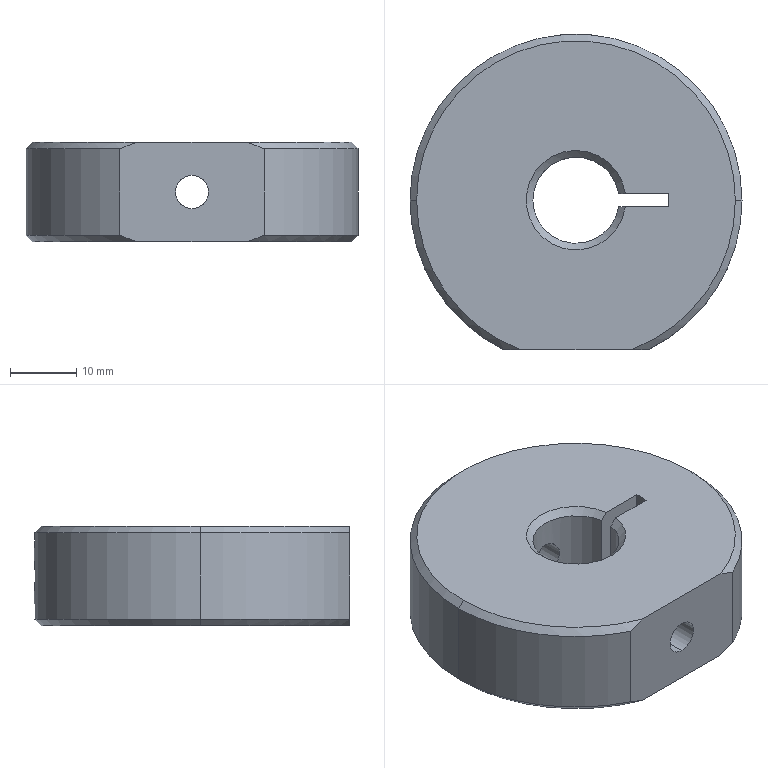Part | STEP file | 11-FG-B01511 | 1 solid | 24 faces | box 50 x 47.5 x 15 mm | volume 25829 mm3 | cylinder 10 | cone 9 | plane 5 | commonest cylinder face diameters 5 x4 50 x3 13 x2 28 x1
STEP:
#1=CARTESIAN_POINT('',(0.,25.,10.));
#2=VERTEX_POINT('',#1);
#3=CARTESIAN_POINT('',(0.,25.,5.));
#4=VERTEX_POINT('',#3);
#5=CARTESIAN_POINT('',(0.,25.,10.));
#6=CARTESIAN_POINT('',(-0.1632,25.,10.));
#7=CARTESIAN_POINT('',(-0.3254,24.998,9.984));
#8=CARTESIAN_POINT('',(-0.648,24.992,9.92));
#9=CARTESIAN_POINT('',(-0.8058,24.987,9.872));
#10=CARTESIAN_POINT('',(-1.107,24.976,9.748));
#11=CARTESIAN_POINT('',(-1.252,24.969,9.67));
#12=CARTESIAN_POINT('',(-1.525,24.954,9.487));
#13=CARTESIAN_POINT('',(-1.651,24.946,9.384));
#14=CARTESIAN_POINT('',(-1.882,24.929,9.154));
#15=CARTESIAN_POINT('',(-1.987,24.921,9.025));
#16=CARTESIAN_POINT('',(-2.169,24.906,8.754));
#17=CARTESIAN_POINT('',(-2.246,24.899,8.61));
#18=CARTESIAN_POINT('',(-2.372,24.887,8.308));
#19=CARTESIAN_POINT('',(-2.42,24.883,8.149));
#20=CARTESIAN_POINT('',(-2.484,24.876,7.829));
#21=CARTESIAN_POINT('',(-2.5,24.875,7.667));
#22=CARTESIAN_POINT('',(-2.5,24.875,7.337));
#23=CARTESIAN_POINT('',(-2.484,24.876,7.174));
#24=CARTESIAN_POINT('',(-2.421,24.883,6.854));
#25=CARTESIAN_POINT('',(-2.373,24.887,6.696));
#26=CARTESIAN_POINT('',(-2.247,24.899,6.393));
#27=CARTESIAN_POINT('',(-2.171,24.906,6.249));
#28=CARTESIAN_POINT('',(-1.99,24.921,5.977));
#29=CARTESIAN_POINT('',(-1.884,24.929,5.849));
#30=CARTESIAN_POINT('',(-1.654,24.946,5.618));
#31=CARTESIAN_POINT('',(-1.528,24.954,5.515));
#32=CARTESIAN_POINT('',(-1.255,24.969,5.332));
#33=CARTESIAN_POINT('',(-1.11,24.976,5.254));
#34=CARTESIAN_POINT('',(-0.6589,24.993,5.067));
#35=CARTESIAN_POINT('',(-0.3305,25.,5.));
#36=CARTESIAN_POINT('',(0.,25.,5.));
#37=B_SPLINE_CURVE_WITH_KNOTS('',3,(#5,#6,#7,#8,#9,#10,#11,#12,#13,#14,#15,#16,#17,#18,#19,#20,#21,#22,#23,#24,#25,#26,#27,#28,#29,#30,#31,#32,#33,#34,#35,#36),.UNSPECIFIED.,.F.,.F.,(4,2,2,2,2,2,2,2,2,2,2,2,2,2,2,4),(0.007821,0.00831,0.008798,0.009287,0.009776,0.01026,0.01075,0.01124,0.01173,0.01222,0.01271,0.0132,0.01369,0.01417,0.01466,0.01564),.UNSPECIFIED.);
#38=EDGE_CURVE('',#2,#4,#37,.T.);
#39=ORIENTED_EDGE('',*,*,#38,.F.);
#40=CARTESIAN_POINT('',(0.,6.5,10.));
#41=VERTEX_POINT('',#40);
#42=CARTESIAN_POINT('',(0.,-22.5,10.));
#43=DIRECTION('',(0.,-1.,0.));
#44=VECTOR('',#43,1000.);
#45=LINE('',#42,#44);
#46=EDGE_CURVE('',#2,#41,#45,.T.);
#47=ORIENTED_EDGE('',*,*,#46,.T.);
#48=CARTESIAN_POINT('',(0.,6.5,5.));
#49=VERTEX_POINT('',#48);
#50=CARTESIAN_POINT('',(0.,6.5,10.));
#51=CARTESIAN_POINT('',(-0.1644,6.5,10.));
#52=CARTESIAN_POINT('',(-0.3308,6.494,9.984));
#53=CARTESIAN_POINT('',(-0.6549,6.469,9.918));
#54=CARTESIAN_POINT('',(-0.8114,6.451,9.87));
#55=CARTESIAN_POINT('',(-1.114,6.406,9.744));
#56=CARTESIAN_POINT('',(-1.259,6.378,9.666));
#57=CARTESIAN_POINT('',(-1.529,6.319,9.485));
#58=CARTESIAN_POINT('',(-1.654,6.287,9.382));
#59=CARTESIAN_POINT('',(-1.885,6.222,9.151));
#60=CARTESIAN_POINT('',(-1.987,6.189,9.025));
#61=CARTESIAN_POINT('',(-2.167,6.129,8.757));
#62=CARTESIAN_POINT('',(-2.245,6.1,8.611));
#63=CARTESIAN_POINT('',(-2.371,6.052,8.309));
#64=CARTESIAN_POINT('',(-2.419,6.033,8.153));
#65=CARTESIAN_POINT('',(-2.483,6.007,7.831));
#66=CARTESIAN_POINT('',(-2.5,6.,7.663));
#67=CARTESIAN_POINT('',(-2.5,6.,7.334));
#68=CARTESIAN_POINT('',(-2.484,6.007,7.17));
#69=CARTESIAN_POINT('',(-2.418,6.033,6.845));
#70=CARTESIAN_POINT('',(-2.37,6.053,6.687));
#71=CARTESIAN_POINT('',(-2.244,6.101,6.386));
#72=CARTESIAN_POINT('',(-2.166,6.129,6.241));
#73=CARTESIAN_POINT('',(-1.984,6.19,5.971));
#74=CARTESIAN_POINT('',(-1.882,6.223,5.846));
#75=CARTESIAN_POINT('',(-1.652,6.288,5.617));
#76=CARTESIAN_POINT('',(-1.525,6.32,5.512));
#77=CARTESIAN_POINT('',(-1.256,6.379,5.332));
#78=CARTESIAN_POINT('',(-1.113,6.406,5.255));
#79=CARTESIAN_POINT('',(-0.8088,6.451,5.129));
#80=CARTESIAN_POINT('',(-0.6508,6.469,5.081));
#81=CARTESIAN_POINT('',(-0.3305,6.494,5.017));
#82=CARTESIAN_POINT('',(-0.1669,6.5,5.));
#83=CARTESIAN_POINT('',(0.,6.5,5.));
#84=B_SPLINE_CURVE_WITH_KNOTS('',3,(#50,#51,#52,#53,#54,#55,#56,#57,#58,#59,#60,#61,#62,#63,#64,#65,#66,#67,#68,#69,#70,#71,#72,#73,#74,#75,#76,#77,#78,#79,#80,#81,#82,#83),.UNSPECIFIED.,.F.,.F.,(4,2,2,2,2,2,2,2,2,2,2,2,2,2,2,2,4),(0.007893,0.008386,0.008879,0.009373,0.009866,0.01036,0.01085,0.01135,0.01184,0.01233,0.01283,0.01332,0.01381,0.0143,0.0148,0.01529,0.01578),.UNSPECIFIED.);
#85=EDGE_CURVE('',#41,#49,#84,.T.);
#86=ORIENTED_EDGE('',*,*,#85,.T.);
#87=CARTESIAN_POINT('',(0.,-22.5,5.));
#88=DIRECTION('',(0.,-1.,0.));
#89=VECTOR('',#88,1000.);
#90=LINE('',#87,#89);
#91=EDGE_CURVE('',#4,#49,#90,.T.);
#92=ORIENTED_EDGE('',*,*,#91,.F.);
#93=EDGE_LOOP('',(#39,#47,#86,#92));
#94=FACE_OUTER_BOUND('',#93,.T.);
#95=CARTESIAN_POINT('',(0.,-22.5,7.5));
#96=DIRECTION('',(0.,-1.,0.));
#97=DIRECTION('',(0.,0.,-1.));
#98=AXIS2_PLACEMENT_3D('',#95,#96,#97);
#99=CYLINDRICAL_SURFACE('',#98,2.5);
#100=ADVANCED_FACE('',(#94),#99,.F.);
#101=CARTESIAN_POINT('',(0.,-6.5,5.));
#102=VERTEX_POINT('',#101);
#103=CARTESIAN_POINT('',(0.,-6.5,10.));
#104=VERTEX_POINT('',#103);
#105=CARTESIAN_POINT('',(0.,-6.5,5.));
#106=CARTESIAN_POINT('',(-0.1669,-6.5,5.));
#107=CARTESIAN_POINT('',(-0.3307,-6.494,5.017));
#108=CARTESIAN_POINT('',(-0.6525,-6.469,5.081));
#109=CARTESIAN_POINT('',(-0.8122,-6.451,5.13));
#110=CARTESIAN_POINT('',(-1.114,-6.406,5.256));
#111=CARTESIAN_POINT('',(-1.257,-6.379,5.333));
#112=CARTESIAN_POINT('',(-1.528,-6.319,5.515));
#113=CARTESIAN_POINT('',(-1.655,-6.287,5.619));
#114=CARTESIAN_POINT('',(-1.997,-6.19,5.962));
#115=CARTESIAN_POINT('',(-2.182,-6.124,6.238));
#116=CARTESIAN_POINT('',(-2.37,-6.053,6.688));
#117=CARTESIAN_POINT('',(-2.419,-6.033,6.847));
#118=CARTESIAN_POINT('',(-2.484,-6.007,7.17));
#119=CARTESIAN_POINT('',(-2.5,-6.,7.334));
#120=CARTESIAN_POINT('',(-2.5,-6.,7.663));
#121=CARTESIAN_POINT('',(-2.483,-6.007,7.831));
#122=CARTESIAN_POINT('',(-2.419,-6.033,8.153));
#123=CARTESIAN_POINT('',(-2.371,-6.053,8.31));
#124=CARTESIAN_POINT('',(-2.244,-6.101,8.614));
#125=CARTESIAN_POINT('',(-2.167,-6.129,8.758));
#126=CARTESIAN_POINT('',(-1.986,-6.19,9.027));
#127=CARTESIAN_POINT('',(-1.882,-6.223,9.154));
#128=CARTESIAN_POINT('',(-1.652,-6.288,9.383));
#129=CARTESIAN_POINT('',(-1.528,-6.319,9.485));
#130=CARTESIAN_POINT('',(-1.258,-6.379,9.667));
#131=CARTESIAN_POINT('',(-1.112,-6.406,9.745));
#132=CARTESIAN_POINT('',(-0.8111,-6.451,9.87));
#133=CARTESIAN_POINT('',(-0.6549,-6.469,9.918));
#134=CARTESIAN_POINT('',(-0.3297,-6.494,9.984));
#135=CARTESIAN_POINT('',(-0.1644,-6.5,10.));
#136=CARTESIAN_POINT('',(0.,-6.5,10.));
#137=B_SPLINE_CURVE_WITH_KNOTS('',3,(#105,#106,#107,#108,#109,#110,#111,#112,#113,#114,#115,#116,#117,#118,#119,#120,#121,#122,#123,#124,#125,#126,#127,#128,#129,#130,#131,#132,#133,#134,#135,#136),.UNSPECIFIED.,.F.,.F.,(4,2,2,2,2,2,2,2,2,2,2,2,2,2,2,4),(0.,0.0004933,0.0009866,0.00148,0.001973,0.00296,0.003453,0.003946,0.00444,0.004933,0.005426,0.00592,0.006413,0.006906,0.0074,0.007893),.UNSPECIFIED.);
#138=EDGE_CURVE('',#102,#104,#137,.T.);
#139=ORIENTED_EDGE('',*,*,#138,.T.);
#140=CARTESIAN_POINT('',(0.,-22.5,10.));
#141=VERTEX_POINT('',#140);
#142=CARTESIAN_POINT('',(0.,-22.5,10.));
#143=DIRECTION('',(0.,-1.,0.));
#144=VECTOR('',#143,1000.);
#145=LINE('',#142,#144);
#146=EDGE_CURVE('',#104,#141,#145,.T.);
#147=ORIENTED_EDGE('',*,*,#146,.T.);
#148=CARTESIAN_POINT('',(0.,-22.5,5.));
#149=VERTEX_POINT('',#148);
#150=CARTESIAN_POINT('',(0.,-22.5,7.5));
#151=DIRECTION('',(0.,-1.,0.));
#152=DIRECTION('',(0.,0.,-1.));
#153=AXIS2_PLACEMENT_3D('',#150,#151,#152);
#154=CIRCLE('',#153,2.5);
#155=EDGE_CURVE('',#141,#149,#154,.T.);
#156=ORIENTED_EDGE('',*,*,#155,.T.);
#157=CARTESIAN_POINT('',(0.,-22.5,5.));
#158=DIRECTION('',(0.,-1.,0.));
#159=VECTOR('',#158,1000.);
#160=LINE('',#157,#159);
#161=EDGE_CURVE('',#102,#149,#160,.T.);
#162=ORIENTED_EDGE('',*,*,#161,.F.);
#163=EDGE_LOOP('',(#139,#147,#156,#162));
#164=FACE_OUTER_BOUND('',#163,.T.);
#165=CARTESIAN_POINT('',(0.,-22.5,7.5));
#166=DIRECTION('',(0.,-1.,0.));
#167=DIRECTION('',(0.,0.,-1.));
#168=AXIS2_PLACEMENT_3D('',#165,#166,#167);
#169=CYLINDRICAL_SURFACE('',#168,2.5);
#170=ADVANCED_FACE('',(#164),#169,.F.);
#171=CARTESIAN_POINT('',(24.,0.,15.));
#172=VERTEX_POINT('',#171);
#173=CARTESIAN_POINT('',(-24.,0.,15.));
#174=VERTEX_POINT('',#173);
#175=CARTESIAN_POINT('',(0.,0.,15.));
#176=DIRECTION('',(0.,0.,1.));
#177=DIRECTION('',(1.,0.,0.));
#178=AXIS2_PLACEMENT_3D('',#175,#176,#177);
#179=CIRCLE('',#178,24.);
#180=EDGE_CURVE('',#172,#174,#179,.T.);
#181=ORIENTED_EDGE('',*,*,#180,.F.);
#182=CARTESIAN_POINT('',(25.,0.,14.));
#183=VERTEX_POINT('',#182);
#184=CARTESIAN_POINT('',(24.,0.,15.));
#185=DIRECTION('',(0.7071,0.,-0.7071));
#186=VECTOR('',#185,1000.);
#187=LINE('',#184,#186);
#188=EDGE_CURVE('',#172,#183,#187,.T.);
#189=ORIENTED_EDGE('',*,*,#188,.T.);
#190=CARTESIAN_POINT('',(-25.,0.,14.));
#191=VERTEX_POINT('',#190);
#192=CARTESIAN_POINT('',(0.,0.,14.));
#193=DIRECTION('',(0.,0.,-1.));
#194=DIRECTION('',(1.,0.,0.));
#195=AXIS2_PLACEMENT_3D('',#192,#193,#194);
#196=CIRCLE('',#195,25.);
#197=EDGE_CURVE('',#191,#183,#196,.T.);
#198=ORIENTED_EDGE('',*,*,#197,.F.);
#199=CARTESIAN_POINT('',(-24.,0.,15.));
#200=DIRECTION('',(-0.7071,0.,-0.7071));
#201=VECTOR('',#200,1000.);
#202=LINE('',#199,#201);
#203=EDGE_CURVE('',#174,#191,#202,.T.);
#204=ORIENTED_EDGE('',*,*,#203,.F.);
#205=EDGE_LOOP('',(#181,#189,#198,#204));
#206=FACE_OUTER_BOUND('',#205,.T.);
#207=CARTESIAN_POINT('',(0.,0.,15.));
#208=DIRECTION('',(0.,0.,-1.));
#209=DIRECTION('',(-1.,0.,0.));
#210=AXIS2_PLACEMENT_3D('',#207,#208,#209);
#211=CONICAL_SURFACE('',#210,24.,0.7854);
#212=ADVANCED_FACE('',(#206),#211,.T.);
#213=CARTESIAN_POINT('',(-8.352,-22.5,15.));
#214=VERTEX_POINT('',#213);
#215=CARTESIAN_POINT('',(0.,0.,15.));
#216=DIRECTION('',(0.,0.,1.));
#217=DIRECTION('',(1.,0.,0.));
#218=AXIS2_PLACEMENT_3D('',#215,#216,#217);
#219=CIRCLE('',#218,24.);
#220=EDGE_CURVE('',#174,#214,#219,.T.);
#221=ORIENTED_EDGE('',*,*,#220,.F.);
#222=ORIENTED_EDGE('',*,*,#203,.T.);
#223=CARTESIAN_POINT('',(-10.897,-22.5,14.));
#224=VERTEX_POINT('',#223);
#225=CARTESIAN_POINT('',(0.,0.,14.));
#226=DIRECTION('',(0.,0.,-1.));
#227=DIRECTION('',(1.,0.,0.));
#228=AXIS2_PLACEMENT_3D('',#225,#226,#227);
#229=CIRCLE('',#228,25.);
#230=EDGE_CURVE('',#224,#191,#229,.T.);
#231=ORIENTED_EDGE('',*,*,#230,.F.);
#232=CARTESIAN_POINT('',(-8.352,-22.5,15.));
#233=CARTESIAN_POINT('',(-9.21,-22.5,14.701));
#234=CARTESIAN_POINT('',(-10.062,-22.5,14.364));
#235=CARTESIAN_POINT('',(-10.897,-22.5,14.));
#236=B_SPLINE_CURVE_WITH_KNOTS('',3,(#232,#233,#234,#235),.UNSPECIFIED.,.F.,.F.,(4,4),(0.06645,0.06918),.UNSPECIFIED.);
#237=EDGE_CURVE('',#214,#224,#236,.T.);
#238=ORIENTED_EDGE('',*,*,#237,.F.);
#239=EDGE_LOOP('',(#221,#222,#231,#238));
#240=FACE_OUTER_BOUND('',#239,.T.);
#241=CARTESIAN_POINT('',(0.,0.,15.));
#242=DIRECTION('',(0.,0.,-1.));
#243=DIRECTION('',(-1.,0.,0.));
#244=AXIS2_PLACEMENT_3D('',#241,#242,#243);
#245=CONICAL_SURFACE('',#244,24.,0.7854);
#246=ADVANCED_FACE('',(#240),#245,.T.);
#247=CARTESIAN_POINT('',(-24.,0.,0.));
#248=VERTEX_POINT('',#247);
#249=CARTESIAN_POINT('',(24.,0.,0.));
#250=VERTEX_POINT('',#249);
#251=CARTESIAN_POINT('',(0.,0.,0.));
#252=DIRECTION('',(0.,0.,-1.));
#253=DIRECTION('',(1.,0.,0.));
#254=AXIS2_PLACEMENT_3D('',#251,#252,#253);
#255=CIRCLE('',#254,24.);
#256=EDGE_CURVE('',#248,#250,#255,.T.);
#257=ORIENTED_EDGE('',*,*,#256,.F.);
#258=CARTESIAN_POINT('',(-25.,0.,1.));
#259=VERTEX_POINT('',#258);
#260=CARTESIAN_POINT('',(-25.,0.,1.));
#261=DIRECTION('',(-0.7071,0.,0.7071));
#262=VECTOR('',#261,1000.);
#263=LINE('',#260,#262);
#264=EDGE_CURVE('',#248,#259,#263,.T.);
#265=ORIENTED_EDGE('',*,*,#264,.T.);
#266=CARTESIAN_POINT('',(25.,0.,1.));
#267=VERTEX_POINT('',#266);
#268=CARTESIAN_POINT('',(0.,0.,1.));
#269=DIRECTION('',(0.,0.,1.));
#270=DIRECTION('',(1.,0.,0.));
#271=AXIS2_PLACEMENT_3D('',#268,#269,#270);
#272=CIRCLE('',#271,25.);
#273=EDGE_CURVE('',#267,#259,#272,.T.);
#274=ORIENTED_EDGE('',*,*,#273,.F.);
#275=CARTESIAN_POINT('',(25.,0.,1.));
#276=DIRECTION('',(0.7071,0.,0.7071));
#277=VECTOR('',#276,1000.);
#278=LINE('',#275,#277);
#279=EDGE_CURVE('',#250,#267,#278,.T.);
#280=ORIENTED_EDGE('',*,*,#279,.F.);
#281=EDGE_LOOP('',(#257,#265,#274,#280));
#282=FACE_OUTER_BOUND('',#281,.T.);
#283=CARTESIAN_POINT('',(0.,0.,1.));
#284=DIRECTION('',(0.,0.,1.));
#285=DIRECTION('',(1.,0.,0.));
#286=AXIS2_PLACEMENT_3D('',#283,#284,#285);
#287=CONICAL_SURFACE('',#286,25.,0.7854);
#288=ADVANCED_FACE('',(#282),#287,.T.);
#289=CARTESIAN_POINT('',(8.352,-22.5,0.));
#290=VERTEX_POINT('',#289);
#291=CARTESIAN_POINT('',(0.,0.,0.));
#292=DIRECTION('',(0.,0.,-1.));
#293=DIRECTION('',(1.,0.,0.));
#294=AXIS2_PLACEMENT_3D('',#291,#292,#293);
#295=CIRCLE('',#294,24.);
#296=EDGE_CURVE('',#250,#290,#295,.T.);
#297=ORIENTED_EDGE('',*,*,#296,.F.);
#298=ORIENTED_EDGE('',*,*,#279,.T.);
#299=CARTESIAN_POINT('',(10.897,-22.5,1.));
#300=VERTEX_POINT('',#299);
#301=CARTESIAN_POINT('',(0.,0.,1.));
#302=DIRECTION('',(0.,0.,1.));
#303=DIRECTION('',(1.,0.,0.));
#304=AXIS2_PLACEMENT_3D('',#301,#302,#303);
#305=CIRCLE('',#304,25.);
#306=EDGE_CURVE('',#300,#267,#305,.T.);
#307=ORIENTED_EDGE('',*,*,#306,.F.);
#308=CARTESIAN_POINT('',(8.352,-22.5,0.));
#309=CARTESIAN_POINT('',(9.21,-22.5,0.2988));
#310=CARTESIAN_POINT('',(10.062,-22.5,0.6359));
#311=CARTESIAN_POINT('',(10.897,-22.5,1.));
#312=B_SPLINE_CURVE_WITH_KNOTS('',3,(#308,#309,#310,#311),.UNSPECIFIED.,.F.,.F.,(4,4),(0.06645,0.06918),.UNSPECIFIED.);
#313=EDGE_CURVE('',#290,#300,#312,.T.);
#314=ORIENTED_EDGE('',*,*,#313,.F.);
#315=EDGE_LOOP('',(#297,#298,#307,#314));
#316=FACE_OUTER_BOUND('',#315,.T.);
#317=CARTESIAN_POINT('',(0.,0.,1.));
#318=DIRECTION('',(0.,0.,1.));
#319=DIRECTION('',(1.,0.,0.));
#320=AXIS2_PLACEMENT_3D('',#317,#318,#319);
#321=CONICAL_SURFACE('',#320,25.,0.7854);
#322=ADVANCED_FACE('',(#316),#321,.T.);
#323=CARTESIAN_POINT('',(-6.5,0.,1.));
#324=VERTEX_POINT('',#323);
#325=CARTESIAN_POINT('',(6.423,1.,1.));
#326=VERTEX_POINT('',#325);
#327=CARTESIAN_POINT('',(0.,0.,1.));
#328=DIRECTION('',(0.,0.,-1.));
#329=DIRECTION('',(1.,0.,0.));
#330=AXIS2_PLACEMENT_3D('',#327,#328,#329);
#331=CIRCLE('',#330,6.5);
#332=EDGE_CURVE('',#324,#326,#331,.T.);
#333=ORIENTED_EDGE('',*,*,#332,.F.);
#334=CARTESIAN_POINT('',(-7.5,0.,0.));
#335=VERTEX_POINT('',#334);
#336=CARTESIAN_POINT('',(-7.5,0.,0.));
#337=DIRECTION('',(-0.7071,0.,-0.7071));
#338=VECTOR('',#337,1000.);
#339=LINE('',#336,#338);
#340=EDGE_CURVE('',#324,#335,#339,.T.);
#341=ORIENTED_EDGE('',*,*,#340,.T.);
#342=CARTESIAN_POINT('',(7.433,1.,0.));
#343=VERTEX_POINT('',#342);
#344=CARTESIAN_POINT('',(0.,0.,0.));
#345=DIRECTION('',(0.,0.,1.));
#346=DIRECTION('',(1.,0.,0.));
#347=AXIS2_PLACEMENT_3D('',#344,#345,#346);
#348=CIRCLE('',#347,7.5);
#349=EDGE_CURVE('',#343,#335,#348,.T.);
#350=ORIENTED_EDGE('',*,*,#349,.F.);
#351=CARTESIAN_POINT('',(6.423,1.,1.));
#352=CARTESIAN_POINT('',(6.595,1.,0.8297));
#353=CARTESIAN_POINT('',(6.767,1.,0.6594));
#354=CARTESIAN_POINT('',(6.939,1.,0.4889));
#355=CARTESIAN_POINT('',(7.104,1.,0.326));
#356=CARTESIAN_POINT('',(7.269,1.,0.163));
#357=CARTESIAN_POINT('',(7.433,1.,0.));
#358=B_SPLINE_CURVE_WITH_KNOTS('',3,(#351,#352,#353,#354,#355,#356,#357),.UNSPECIFIED.,.F.,.F.,(4,3,4),(0.001962,0.002688,0.003383),.UNSPECIFIED.);
#359=EDGE_CURVE('',#326,#343,#358,.T.);
#360=ORIENTED_EDGE('',*,*,#359,.F.);
#361=EDGE_LOOP('',(#333,#341,#350,#360));
#362=FACE_OUTER_BOUND('',#361,.T.);
#363=CARTESIAN_POINT('',(0.,0.,0.));
#364=DIRECTION('',(0.,0.,-1.));
#365=DIRECTION('',(-1.,0.,0.));
#366=AXIS2_PLACEMENT_3D('',#363,#364,#365);
#367=CONICAL_SURFACE('',#366,7.5,0.7854);
#368=ADVANCED_FACE('',(#362),#367,.F.);
#369=CARTESIAN_POINT('',(0.,6.5,5.));
#370=CARTESIAN_POINT('',(0.1669,6.5,5.));
#371=CARTESIAN_POINT('',(0.3307,6.494,5.017));
#372=CARTESIAN_POINT('',(0.6525,6.469,5.081));
#373=CARTESIAN_POINT('',(0.8122,6.451,5.13));
#374=CARTESIAN_POINT('',(1.114,6.406,5.256));
#375=CARTESIAN_POINT('',(1.257,6.379,5.333));
#376=CARTESIAN_POINT('',(1.528,6.319,5.515));
#377=CARTESIAN_POINT('',(1.655,6.287,5.619));
#378=CARTESIAN_POINT('',(1.997,6.19,5.962));
#379=CARTESIAN_POINT('',(2.182,6.124,6.238));
#380=CARTESIAN_POINT('',(2.37,6.053,6.688));
#381=CARTESIAN_POINT('',(2.419,6.033,6.847));
#382=CARTESIAN_POINT('',(2.484,6.007,7.17));
#383=CARTESIAN_POINT('',(2.5,6.,7.334));
#384=CARTESIAN_POINT('',(2.5,6.,7.663));
#385=CARTESIAN_POINT('',(2.483,6.007,7.831));
#386=CARTESIAN_POINT('',(2.419,6.033,8.153));
#387=CARTESIAN_POINT('',(2.371,6.053,8.31));
#388=CARTESIAN_POINT('',(2.244,6.101,8.614));
#389=CARTESIAN_POINT('',(2.167,6.129,8.758));
#390=CARTESIAN_POINT('',(1.986,6.19,9.027));
#391=CARTESIAN_POINT('',(1.882,6.223,9.154));
#392=CARTESIAN_POINT('',(1.652,6.288,9.383));
#393=CARTESIAN_POINT('',(1.528,6.319,9.485));
#394=CARTESIAN_POINT('',(1.258,6.379,9.667));
#395=CARTESIAN_POINT('',(1.112,6.406,9.745));
#396=CARTESIAN_POINT('',(0.8111,6.451,9.87));
#397=CARTESIAN_POINT('',(0.6549,6.469,9.918));
#398=CARTESIAN_POINT('',(0.3297,6.494,9.984));
#399=CARTESIAN_POINT('',(0.1644,6.5,10.));
#400=CARTESIAN_POINT('',(0.,6.5,10.));
#401=B_SPLINE_CURVE_WITH_KNOTS('',3,(#369,#370,#371,#372,#373,#374,#375,#376,#377,#378,#379,#380,#381,#382,#383,#384,#385,#386,#387,#388,#389,#390,#391,#392,#393,#394,#395,#396,#397,#398,#399,#400),.UNSPECIFIED.,.F.,.F.,(4,2,2,2,2,2,2,2,2,2,2,2,2,2,2,4),(0.,0.0004933,0.0009866,0.00148,0.001973,0.00296,0.003453,0.003946,0.00444,0.004933,0.005426,0.00592,0.006413,0.006906,0.0074,0.007893),.UNSPECIFIED.);
#402=EDGE_CURVE('',#49,#41,#401,.T.);
#403=ORIENTED_EDGE('',*,*,#402,.F.);
#404=ORIENTED_EDGE('',*,*,#85,.F.);
#405=EDGE_LOOP('',(#403,#404));
#406=FACE_BOUND('',#405,.T.);
#407=CARTESIAN_POINT('',(6.423,1.,14.));
#408=VERTEX_POINT('',#407);
#409=CARTESIAN_POINT('',(-6.5,0.,14.));
#410=VERTEX_POINT('',#409);
#411=CARTESIAN_POINT('',(0.,0.,14.));
#412=DIRECTION('',(0.,0.,1.));
#413=DIRECTION('',(1.,0.,0.));
#414=AXIS2_PLACEMENT_3D('',#411,#412,#413);
#415=CIRCLE('',#414,6.5);
#416=EDGE_CURVE('',#408,#410,#415,.T.);
#417=ORIENTED_EDGE('',*,*,#416,.T.);
#418=CARTESIAN_POINT('',(-6.5,0.,15.));
#419=DIRECTION('',(0.,0.,-1.));
#420=VECTOR('',#419,1000.);
#421=LINE('',#418,#420);
#422=EDGE_CURVE('',#410,#324,#421,.T.);
#423=ORIENTED_EDGE('',*,*,#422,.T.);
#424=ORIENTED_EDGE('',*,*,#332,.T.);
#425=CARTESIAN_POINT('',(6.423,1.,19.));
#426=DIRECTION('',(0.,0.,-1.));
#427=VECTOR('',#426,1000.);
#428=LINE('',#425,#427);
#429=EDGE_CURVE('',#408,#326,#428,.T.);
#430=ORIENTED_EDGE('',*,*,#429,.F.);
#431=EDGE_LOOP('',(#417,#423,#424,#430));
#432=FACE_OUTER_BOUND('',#431,.T.);
#433=CARTESIAN_POINT('',(0.,0.,15.));
#434=DIRECTION('',(0.,0.,-1.));
#435=DIRECTION('',(-1.,0.,0.));
#436=AXIS2_PLACEMENT_3D('',#433,#434,#435);
#437=CYLINDRICAL_SURFACE('',#436,6.5);
#438=ADVANCED_FACE('',(#406,#432),#437,.F.);
#439=CARTESIAN_POINT('',(0.,25.,5.));
#440=CARTESIAN_POINT('',(0.1653,25.,5.));
#441=CARTESIAN_POINT('',(0.3278,24.998,5.016));
#442=CARTESIAN_POINT('',(0.6475,24.992,5.08));
#443=CARTESIAN_POINT('',(0.8063,24.987,5.128));
#444=CARTESIAN_POINT('',(1.109,24.976,5.253));
#445=CARTESIAN_POINT('',(1.253,24.969,5.33));
#446=CARTESIAN_POINT('',(1.524,24.954,5.512));
#447=CARTESIAN_POINT('',(1.653,24.946,5.617));
#448=CARTESIAN_POINT('',(1.883,24.929,5.848));
#449=CARTESIAN_POINT('',(1.987,24.921,5.974));
#450=CARTESIAN_POINT('',(2.17,24.906,6.247));
#451=CARTESIAN_POINT('',(2.247,24.899,6.392));
#452=CARTESIAN_POINT('',(2.372,24.887,6.693));
#453=CARTESIAN_POINT('',(2.42,24.883,6.851));
#454=CARTESIAN_POINT('',(2.484,24.876,7.174));
#455=CARTESIAN_POINT('',(2.5,24.875,7.336));
#456=CARTESIAN_POINT('',(2.5,24.875,7.662));
#457=CARTESIAN_POINT('',(2.484,24.876,7.828));
#458=CARTESIAN_POINT('',(2.42,24.883,8.149));
#459=CARTESIAN_POINT('',(2.373,24.887,8.305));
#460=CARTESIAN_POINT('',(2.247,24.899,8.607));
#461=CARTESIAN_POINT('',(2.169,24.906,8.754));
#462=CARTESIAN_POINT('',(1.988,24.921,9.025));
#463=CARTESIAN_POINT('',(1.885,24.929,9.151));
#464=CARTESIAN_POINT('',(1.651,24.946,9.384));
#465=CARTESIAN_POINT('',(1.525,24.954,9.488));
#466=CARTESIAN_POINT('',(1.254,24.969,9.669));
#467=CARTESIAN_POINT('',(1.108,24.976,9.747));
#468=CARTESIAN_POINT('',(0.8054,24.987,9.872));
#469=CARTESIAN_POINT('',(0.6496,24.992,9.92));
#470=CARTESIAN_POINT('',(0.329,24.998,9.984));
#471=CARTESIAN_POINT('',(0.1632,25.,10.));
#472=CARTESIAN_POINT('',(0.,25.,10.));
#473=B_SPLINE_CURVE_WITH_KNOTS('',3,(#439,#440,#441,#442,#443,#444,#445,#446,#447,#448,#449,#450,#451,#452,#453,#454,#455,#456,#457,#458,#459,#460,#461,#462,#463,#464,#465,#466,#467,#468,#469,#470,#471,#472),.UNSPECIFIED.,.F.,.F.,(4,2,2,2,2,2,2,2,2,2,2,2,2,2,2,2,4),(0.,0.0004888,0.0009776,0.001466,0.001955,0.002444,0.002933,0.003422,0.003911,0.004399,0.004888,0.005377,0.005866,0.006355,0.006843,0.007332,0.007821),.UNSPECIFIED.);
#474=EDGE_CURVE('',#4,#2,#473,.T.);
#475=ORIENTED_EDGE('',*,*,#474,.T.);
#476=ORIENTED_EDGE('',*,*,#38,.T.);
#477=EDGE_LOOP('',(#475,#476));
#478=FACE_BOUND('',#477,.T.);
#479=ORIENTED_EDGE('',*,*,#197,.T.);
#480=CARTESIAN_POINT('',(25.,0.,15.));
#481=DIRECTION('',(0.,0.,-1.));
#482=VECTOR('',#481,1000.);
#483=LINE('',#480,#482);
#484=EDGE_CURVE('',#183,#267,#483,.T.);
#485=ORIENTED_EDGE('',*,*,#484,.T.);
#486=ORIENTED_EDGE('',*,*,#273,.T.);
#487=CARTESIAN_POINT('',(-25.,0.,15.));
#488=DIRECTION('',(0.,0.,-1.));
#489=VECTOR('',#488,1000.);
#490=LINE('',#487,#489);
#491=EDGE_CURVE('',#191,#259,#490,.T.);
#492=ORIENTED_EDGE('',*,*,#491,.F.);
#493=EDGE_LOOP('',(#479,#485,#486,#492));
#494=FACE_OUTER_BOUND('',#493,.T.);
#495=CARTESIAN_POINT('',(0.,0.,15.));
#496=DIRECTION('',(0.,0.,-1.));
#497=DIRECTION('',(-1.,0.,0.));
#498=AXIS2_PLACEMENT_3D('',#495,#496,#497);
#499=CYLINDRICAL_SURFACE('',#498,25.);
#500=ADVANCED_FACE('',(#478,#494),#499,.T.);
#501=ORIENTED_EDGE('',*,*,#230,.T.);
#502=ORIENTED_EDGE('',*,*,#491,.T.);
#503=CARTESIAN_POINT('',(-10.897,-22.5,1.));
#504=VERTEX_POINT('',#503);
#505=CARTESIAN_POINT('',(0.,0.,1.));
#506=DIRECTION('',(0.,0.,1.));
#507=DIRECTION('',(1.,0.,0.));
#508=AXIS2_PLACEMENT_3D('',#505,#506,#507);
#509=CIRCLE('',#508,25.);
#510=EDGE_CURVE('',#259,#504,#509,.T.);
#511=ORIENTED_EDGE('',*,*,#510,.T.);
#512=CARTESIAN_POINT('',(-10.897,-22.5,15.));
#513=DIRECTION('',(0.,0.,1.));
#514=VECTOR('',#513,1000.);
#515=LINE('',#512,#514);
#516=EDGE_CURVE('',#504,#224,#515,.T.);
#517=ORIENTED_EDGE('',*,*,#516,.T.);
#518=EDGE_LOOP('',(#501,#502,#511,#517));
#519=FACE_OUTER_BOUND('',#518,.T.);
#520=CARTESIAN_POINT('',(0.,0.,15.));
#521=DIRECTION('',(0.,0.,-1.));
#522=DIRECTION('',(-1.,0.,0.));
#523=AXIS2_PLACEMENT_3D('',#520,#521,#522);
#524=CYLINDRICAL_SURFACE('',#523,25.);
#525=ADVANCED_FACE('',(#519),#524,.T.);
#526=ORIENTED_EDGE('',*,*,#313,.T.);
#527=CARTESIAN_POINT('',(10.897,-22.5,14.));
#528=VERTEX_POINT('',#527);
#529=CARTESIAN_POINT('',(10.897,-22.5,15.));
#530=DIRECTION('',(0.,0.,-1.));
#531=VECTOR('',#530,1000.);
#532=LINE('',#529,#531);
#533=EDGE_CURVE('',#528,#300,#532,.T.);
#534=ORIENTED_EDGE('',*,*,#533,.F.);
#535=CARTESIAN_POINT('',(8.352,-22.5,15.));
#536=VERTEX_POINT('',#535);
#537=CARTESIAN_POINT('',(10.897,-22.5,14.));
#538=CARTESIAN_POINT('',(10.061,-22.5,14.365));
#539=CARTESIAN_POINT('',(9.213,-22.5,14.7));
#540=CARTESIAN_POINT('',(8.352,-22.5,15.));
#541=B_SPLINE_CURVE_WITH_KNOTS('',3,(#537,#538,#539,#540),.UNSPECIFIED.,.F.,.F.,(4,4),(0.04668,0.04942),.UNSPECIFIED.);
#542=EDGE_CURVE('',#528,#536,#541,.T.);
#543=ORIENTED_EDGE('',*,*,#542,.T.);
#544=CARTESIAN_POINT('',(-21.698,-22.5,15.));
#545=DIRECTION('',(-1.,0.,0.));
#546=VECTOR('',#545,1000.);
#547=LINE('',#544,#546);
#548=EDGE_CURVE('',#536,#214,#547,.T.);
#549=ORIENTED_EDGE('',*,*,#548,.T.);
#550=ORIENTED_EDGE('',*,*,#237,.T.);
#551=ORIENTED_EDGE('',*,*,#516,.F.);
#552=CARTESIAN_POINT('',(-8.352,-22.5,0.));
#553=VERTEX_POINT('',#552);
#554=CARTESIAN_POINT('',(-10.897,-22.5,1.));
#555=CARTESIAN_POINT('',(-10.061,-22.5,0.6355));
#556=CARTESIAN_POINT('',(-9.213,-22.5,0.2998));
#557=CARTESIAN_POINT('',(-8.352,-22.5,0.));
#558=B_SPLINE_CURVE_WITH_KNOTS('',3,(#554,#555,#556,#557),.UNSPECIFIED.,.F.,.F.,(4,4),(0.04668,0.04942),.UNSPECIFIED.);
#559=EDGE_CURVE('',#504,#553,#558,.T.);
#560=ORIENTED_EDGE('',*,*,#559,.T.);
#561=CARTESIAN_POINT('',(-21.698,-22.5,0.));
#562=DIRECTION('',(-1.,0.,0.));
#563=VECTOR('',#562,1000.);
#564=LINE('',#561,#563);
#565=EDGE_CURVE('',#290,#553,#564,.T.);
#566=ORIENTED_EDGE('',*,*,#565,.F.);
#567=EDGE_LOOP('',(#526,#534,#543,#549,#550,#551,#560,#566));
#568=FACE_OUTER_BOUND('',#567,.T.);
#569=CARTESIAN_POINT('',(0.,-22.5,7.5));
#570=DIRECTION('',(0.,-1.,0.));
#571=DIRECTION('',(0.,0.,-1.));
#572=AXIS2_PLACEMENT_3D('',#569,#570,#571);
#573=CIRCLE('',#572,2.5);
#574=EDGE_CURVE('',#149,#141,#573,.T.);
#575=ORIENTED_EDGE('',*,*,#574,.F.);
#576=ORIENTED_EDGE('',*,*,#155,.F.);
#577=EDGE_LOOP('',(#575,#576));
#578=FACE_BOUND('',#577,.T.);
#579=CARTESIAN_POINT('',(-21.698,-22.5,0.));
#580=DIRECTION('',(0.,1.,0.));
#581=DIRECTION('',(0.,0.,1.));
#582=AXIS2_PLACEMENT_3D('',#579,#580,#581);
#583=PLANE('',#582);
#584=ADVANCED_FACE('',(#568,#578),#583,.F.);
#585=CARTESIAN_POINT('',(7.433,-1.,15.));
#586=VERTEX_POINT('',#585);
#587=CARTESIAN_POINT('',(13.964,-1.,15.));
#588=VERTEX_POINT('',#587);
#589=CARTESIAN_POINT('',(0.,-1.,15.));
#590=DIRECTION('',(1.,0.,0.));
#591=VECTOR('',#590,1000.);
#592=LINE('',#589,#591);
#593=EDGE_CURVE('',#586,#588,#592,.T.);
#594=ORIENTED_EDGE('',*,*,#593,.F.);
#595=CARTESIAN_POINT('',(7.433,1.,15.));
#596=VERTEX_POINT('',#595);
#597=CARTESIAN_POINT('',(0.,0.,15.));
#598=DIRECTION('',(0.,0.,-1.));
#599=DIRECTION('',(1.,0.,0.));
#600=AXIS2_PLACEMENT_3D('',#597,#598,#599);
#601=CIRCLE('',#600,7.5);
#602=EDGE_CURVE('',#586,#596,#601,.T.);
#603=ORIENTED_EDGE('',*,*,#602,.T.);
#604=CARTESIAN_POINT('',(13.964,1.,15.));
#605=VERTEX_POINT('',#604);
#606=CARTESIAN_POINT('',(0.,1.,15.));
#607=DIRECTION('',(-1.,0.,0.));
#608=VECTOR('',#607,1000.);
#609=LINE('',#606,#608);
#610=EDGE_CURVE('',#605,#596,#609,.T.);
#611=ORIENTED_EDGE('',*,*,#610,.F.);
#612=CARTESIAN_POINT('',(0.,0.,15.));
#613=DIRECTION('',(0.,0.,1.));
#614=DIRECTION('',(1.,0.,0.));
#615=AXIS2_PLACEMENT_3D('',#612,#613,#614);
#616=CIRCLE('',#615,14.);
#617=EDGE_CURVE('',#588,#605,#616,.T.);
#618=ORIENTED_EDGE('',*,*,#617,.F.);
#619=EDGE_LOOP('',(#594,#603,#611,#618));
#620=FACE_BOUND('',#619,.T.);
#621=ORIENTED_EDGE('',*,*,#548,.F.);
#622=CARTESIAN_POINT('',(0.,0.,15.));
#623=DIRECTION('',(0.,0.,1.));
#624=DIRECTION('',(1.,0.,0.));
#625=AXIS2_PLACEMENT_3D('',#622,#623,#624);
#626=CIRCLE('',#625,24.);
#627=EDGE_CURVE('',#536,#172,#626,.T.);
#628=ORIENTED_EDGE('',*,*,#627,.T.);
#629=ORIENTED_EDGE('',*,*,#180,.T.);
#630=ORIENTED_EDGE('',*,*,#220,.T.);
#631=EDGE_LOOP('',(#621,#628,#629,#630));
#632=FACE_OUTER_BOUND('',#631,.T.);
#633=CARTESIAN_POINT('',(0.,0.,15.));
#634=DIRECTION('',(0.,0.,1.));
#635=DIRECTION('',(1.,0.,0.));
#636=AXIS2_PLACEMENT_3D('',#633,#634,#635);
#637=PLANE('',#636);
#638=ADVANCED_FACE('',(#620,#632),#637,.T.);
#639=ORIENTED_EDGE('',*,*,#349,.T.);
#640=CARTESIAN_POINT('',(7.433,-1.,0.));
#641=VERTEX_POINT('',#640);
#642=CARTESIAN_POINT('',(0.,0.,0.));
#643=DIRECTION('',(0.,0.,1.));
#644=DIRECTION('',(1.,0.,0.));
#645=AXIS2_PLACEMENT_3D('',#642,#643,#644);
#646=CIRCLE('',#645,7.5);
#647=EDGE_CURVE('',#335,#641,#646,.T.);
#648=ORIENTED_EDGE('',*,*,#647,.T.);
#649=CARTESIAN_POINT('',(13.964,-1.,0.));
#650=VERTEX_POINT('',#649);
#651=CARTESIAN_POINT('',(6.423,-1.,0.));
#652=DIRECTION('',(-1.,0.,0.));
#653=VECTOR('',#652,1000.);
#654=LINE('',#651,#653);
#655=EDGE_CURVE('',#650,#641,#654,.T.);
#656=ORIENTED_EDGE('',*,*,#655,.F.);
#657=CARTESIAN_POINT('',(13.964,1.,0.));
#658=VERTEX_POINT('',#657);
#659=CARTESIAN_POINT('',(0.,0.,0.));
#660=DIRECTION('',(0.,0.,-1.));
#661=DIRECTION('',(-1.,0.,0.));
#662=AXIS2_PLACEMENT_3D('',#659,#660,#661);
#663=CIRCLE('',#662,14.);
#664=EDGE_CURVE('',#658,#650,#663,.T.);
#665=ORIENTED_EDGE('',*,*,#664,.F.);
#666=CARTESIAN_POINT('',(6.423,1.,0.));
#667=DIRECTION('',(1.,0.,0.));
#668=VECTOR('',#667,1000.);
#669=LINE('',#666,#668);
#670=EDGE_CURVE('',#343,#658,#669,.T.);
#671=ORIENTED_EDGE('',*,*,#670,.F.);
#672=EDGE_LOOP('',(#639,#648,#656,#665,#671));
#673=FACE_BOUND('',#672,.T.);
#674=CARTESIAN_POINT('',(0.,0.,0.));
#675=DIRECTION('',(0.,0.,-1.));
#676=DIRECTION('',(1.,0.,0.));
#677=AXIS2_PLACEMENT_3D('',#674,#675,#676);
#678=CIRCLE('',#677,24.);
#679=EDGE_CURVE('',#553,#248,#678,.T.);
#680=ORIENTED_EDGE('',*,*,#679,.T.);
#681=ORIENTED_EDGE('',*,*,#256,.T.);
#682=ORIENTED_EDGE('',*,*,#296,.T.);
#683=ORIENTED_EDGE('',*,*,#565,.T.);
#684=EDGE_LOOP('',(#680,#681,#682,#683));
#685=FACE_OUTER_BOUND('',#684,.T.);
#686=CARTESIAN_POINT('',(0.,0.,0.));
#687=DIRECTION('',(0.,0.,1.));
#688=DIRECTION('',(1.,0.,0.));
#689=AXIS2_PLACEMENT_3D('',#686,#687,#688);
#690=PLANE('',#689);
#691=ADVANCED_FACE('',(#673,#685),#690,.F.);
#692=ORIENTED_EDGE('',*,*,#484,.F.);
#693=CARTESIAN_POINT('',(0.,0.,14.));
#694=DIRECTION('',(0.,0.,-1.));
#695=DIRECTION('',(1.,0.,0.));
#696=AXIS2_PLACEMENT_3D('',#693,#694,#695);
#697=CIRCLE('',#696,25.);
#698=EDGE_CURVE('',#183,#528,#697,.T.);
#699=ORIENTED_EDGE('',*,*,#698,.T.);
#700=ORIENTED_EDGE('',*,*,#533,.T.);
#701=ORIENTED_EDGE('',*,*,#306,.T.);
#702=EDGE_LOOP('',(#692,#699,#700,#701));
#703=FACE_OUTER_BOUND('',#702,.T.);
#704=CARTESIAN_POINT('',(0.,0.,15.));
#705=DIRECTION('',(0.,0.,-1.));
#706=DIRECTION('',(-1.,0.,0.));
#707=AXIS2_PLACEMENT_3D('',#704,#705,#706);
#708=CYLINDRICAL_SURFACE('',#707,25.);
#709=ADVANCED_FACE('',(#703),#708,.T.);
#710=ORIENTED_EDGE('',*,*,#422,.F.);
#711=CARTESIAN_POINT('',(6.423,-1.,14.));
#712=VERTEX_POINT('',#711);
#713=CARTESIAN_POINT('',(0.,0.,14.));
#714=DIRECTION('',(0.,0.,1.));
#715=DIRECTION('',(1.,0.,0.));
#716=AXIS2_PLACEMENT_3D('',#713,#714,#715);
#717=CIRCLE('',#716,6.5);
#718=EDGE_CURVE('',#410,#712,#717,.T.);
#719=ORIENTED_EDGE('',*,*,#718,.T.);
#720=CARTESIAN_POINT('',(6.423,-1.,1.));
#721=VERTEX_POINT('',#720);
#722=CARTESIAN_POINT('',(6.423,-1.,19.));
#723=DIRECTION('',(0.,0.,-1.));
#724=VECTOR('',#723,1000.);
#725=LINE('',#722,#724);
#726=EDGE_CURVE('',#712,#721,#725,.T.);
#727=ORIENTED_EDGE('',*,*,#726,.T.);
#728=CARTESIAN_POINT('',(0.,0.,1.));
#729=DIRECTION('',(0.,0.,-1.));
#730=DIRECTION('',(1.,0.,0.));
#731=AXIS2_PLACEMENT_3D('',#728,#729,#730);
#732=CIRCLE('',#731,6.5);
#733=EDGE_CURVE('',#721,#324,#732,.T.);
#734=ORIENTED_EDGE('',*,*,#733,.T.);
#735=EDGE_LOOP('',(#710,#719,#727,#734));
#736=FACE_OUTER_BOUND('',#735,.T.);
#737=ORIENTED_EDGE('',*,*,#138,.F.);
#738=CARTESIAN_POINT('',(0.,-6.5,10.));
#739=CARTESIAN_POINT('',(0.1644,-6.5,10.));
#740=CARTESIAN_POINT('',(0.3308,-6.494,9.984));
#741=CARTESIAN_POINT('',(0.6549,-6.469,9.918));
#742=CARTESIAN_POINT('',(0.8114,-6.451,9.87));
#743=CARTESIAN_POINT('',(1.114,-6.406,9.744));
#744=CARTESIAN_POINT('',(1.259,-6.378,9.666));
#745=CARTESIAN_POINT('',(1.529,-6.319,9.485));
#746=CARTESIAN_POINT('',(1.654,-6.287,9.382));
#747=CARTESIAN_POINT('',(1.885,-6.222,9.151));
#748=CARTESIAN_POINT('',(1.987,-6.189,9.025));
#749=CARTESIAN_POINT('',(2.167,-6.129,8.757));
#750=CARTESIAN_POINT('',(2.245,-6.1,8.611));
#751=CARTESIAN_POINT('',(2.371,-6.052,8.309));
#752=CARTESIAN_POINT('',(2.419,-6.033,8.153));
#753=CARTESIAN_POINT('',(2.483,-6.007,7.831));
#754=CARTESIAN_POINT('',(2.5,-6.,7.663));
#755=CARTESIAN_POINT('',(2.5,-6.,7.334));
#756=CARTESIAN_POINT('',(2.484,-6.007,7.17));
#757=CARTESIAN_POINT('',(2.418,-6.033,6.845));
#758=CARTESIAN_POINT('',(2.37,-6.053,6.687));
#759=CARTESIAN_POINT('',(2.244,-6.101,6.386));
#760=CARTESIAN_POINT('',(2.166,-6.129,6.241));
#761=CARTESIAN_POINT('',(1.984,-6.19,5.971));
#762=CARTESIAN_POINT('',(1.882,-6.223,5.846));
#763=CARTESIAN_POINT('',(1.652,-6.288,5.617));
#764=CARTESIAN_POINT('',(1.525,-6.32,5.512));
#765=CARTESIAN_POINT('',(1.256,-6.379,5.332));
#766=CARTESIAN_POINT('',(1.113,-6.406,5.255));
#767=CARTESIAN_POINT('',(0.8088,-6.451,5.129));
#768=CARTESIAN_POINT('',(0.6508,-6.469,5.081));
#769=CARTESIAN_POINT('',(0.3305,-6.494,5.017));
#770=CARTESIAN_POINT('',(0.1669,-6.5,5.));
#771=CARTESIAN_POINT('',(0.,-6.5,5.));
#772=B_SPLINE_CURVE_WITH_KNOTS('',3,(#738,#739,#740,#741,#742,#743,#744,#745,#746,#747,#748,#749,#750,#751,#752,#753,#754,#755,#756,#757,#758,#759,#760,#761,#762,#763,#764,#765,#766,#767,#768,#769,#770,#771),.UNSPECIFIED.,.F.,.F.,(4,2,2,2,2,2,2,2,2,2,2,2,2,2,2,2,4),(0.007893,0.008386,0.008879,0.009373,0.009866,0.01036,0.01085,0.01135,0.01184,0.01233,0.01283,0.01332,0.01381,0.0143,0.0148,0.01529,0.01578),.UNSPECIFIED.);
#773=EDGE_CURVE('',#104,#102,#772,.T.);
#774=ORIENTED_EDGE('',*,*,#773,.F.);
#775=EDGE_LOOP('',(#737,#774));
#776=FACE_BOUND('',#775,.T.);
#777=CARTESIAN_POINT('',(0.,0.,15.));
#778=DIRECTION('',(0.,0.,-1.));
#779=DIRECTION('',(-1.,0.,0.));
#780=AXIS2_PLACEMENT_3D('',#777,#778,#779);
#781=CYLINDRICAL_SURFACE('',#780,6.5);
#782=ADVANCED_FACE('',(#736,#776),#781,.F.);
#783=ORIENTED_EDGE('',*,*,#340,.F.);
#784=ORIENTED_EDGE('',*,*,#733,.F.);
#785=CARTESIAN_POINT('',(7.433,-1.,0.));
#786=CARTESIAN_POINT('',(7.269,-1.,0.163));
#787=CARTESIAN_POINT('',(7.104,-1.,0.326));
#788=CARTESIAN_POINT('',(6.939,-1.,0.4889));
#789=CARTESIAN_POINT('',(6.767,-1.,0.6594));
#790=CARTESIAN_POINT('',(6.595,-1.,0.8297));
#791=CARTESIAN_POINT('',(6.423,-1.,1.));
#792=B_SPLINE_CURVE_WITH_KNOTS('',3,(#785,#786,#787,#788,#789,#790,#791),.UNSPECIFIED.,.F.,.F.,(4,3,4),(0.001994,0.002688,0.003415),.UNSPECIFIED.);
#793=EDGE_CURVE('',#641,#721,#792,.T.);
#794=ORIENTED_EDGE('',*,*,#793,.F.);
#795=ORIENTED_EDGE('',*,*,#647,.F.);
#796=EDGE_LOOP('',(#783,#784,#794,#795));
#797=FACE_OUTER_BOUND('',#796,.T.);
#798=CARTESIAN_POINT('',(0.,0.,0.));
#799=DIRECTION('',(0.,0.,-1.));
#800=DIRECTION('',(-1.,0.,0.));
#801=AXIS2_PLACEMENT_3D('',#798,#799,#800);
#802=CONICAL_SURFACE('',#801,7.5,0.7854);
#803=ADVANCED_FACE('',(#797),#802,.F.);
#804=CARTESIAN_POINT('',(6.423,-1.,14.));
#805=CARTESIAN_POINT('',(6.466,-1.,14.043));
#806=CARTESIAN_POINT('',(6.51,-1.,14.086));
#807=CARTESIAN_POINT('',(6.553,-1.,14.129));
#808=CARTESIAN_POINT('',(6.847,-1.,14.419));
#809=CARTESIAN_POINT('',(7.14,-1.,14.71));
#810=CARTESIAN_POINT('',(7.433,-1.,15.));
#811=B_SPLINE_CURVE_WITH_KNOTS('',3,(#804,#805,#806,#807,#808,#809,#810),.UNSPECIFIED.,.F.,.F.,(4,3,4),(0.002505,0.002688,0.003926),.UNSPECIFIED.);
#812=EDGE_CURVE('',#712,#586,#811,.T.);
#813=ORIENTED_EDGE('',*,*,#812,.F.);
#814=ORIENTED_EDGE('',*,*,#718,.F.);
#815=ORIENTED_EDGE('',*,*,#416,.F.);
#816=CARTESIAN_POINT('',(7.433,1.,15.));
#817=CARTESIAN_POINT('',(7.14,1.,14.71));
#818=CARTESIAN_POINT('',(6.847,1.,14.419));
#819=CARTESIAN_POINT('',(6.553,1.,14.129));
#820=CARTESIAN_POINT('',(6.51,1.,14.086));
#821=CARTESIAN_POINT('',(6.466,1.,14.043));
#822=CARTESIAN_POINT('',(6.423,1.,14.));
#823=B_SPLINE_CURVE_WITH_KNOTS('',3,(#816,#817,#818,#819,#820,#821,#822),.UNSPECIFIED.,.F.,.F.,(4,3,4),(0.00145,0.002688,0.002872),.UNSPECIFIED.);
#824=EDGE_CURVE('',#596,#408,#823,.T.);
#825=ORIENTED_EDGE('',*,*,#824,.F.);
#826=ORIENTED_EDGE('',*,*,#602,.F.);
#827=EDGE_LOOP('',(#813,#814,#815,#825,#826));
#828=FACE_OUTER_BOUND('',#827,.T.);
#829=CARTESIAN_POINT('',(0.,0.,14.));
#830=DIRECTION('',(0.,0.,1.));
#831=DIRECTION('',(1.,0.,0.));
#832=AXIS2_PLACEMENT_3D('',#829,#830,#831);
#833=CONICAL_SURFACE('',#832,6.5,0.7854);
#834=ADVANCED_FACE('',(#828),#833,.F.);
#835=ORIENTED_EDGE('',*,*,#264,.F.);
#836=ORIENTED_EDGE('',*,*,#679,.F.);
#837=ORIENTED_EDGE('',*,*,#559,.F.);
#838=ORIENTED_EDGE('',*,*,#510,.F.);
#839=EDGE_LOOP('',(#835,#836,#837,#838));
#840=FACE_OUTER_BOUND('',#839,.T.);
#841=CARTESIAN_POINT('',(0.,0.,1.));
#842=DIRECTION('',(0.,0.,1.));
#843=DIRECTION('',(1.,0.,0.));
#844=AXIS2_PLACEMENT_3D('',#841,#842,#843);
#845=CONICAL_SURFACE('',#844,25.,0.7854);
#846=ADVANCED_FACE('',(#840),#845,.T.);
#847=ORIENTED_EDGE('',*,*,#188,.F.);
#848=ORIENTED_EDGE('',*,*,#627,.F.);
#849=ORIENTED_EDGE('',*,*,#542,.F.);
#850=ORIENTED_EDGE('',*,*,#698,.F.);
#851=EDGE_LOOP('',(#847,#848,#849,#850));
#852=FACE_OUTER_BOUND('',#851,.T.);
#853=CARTESIAN_POINT('',(0.,0.,15.));
#854=DIRECTION('',(0.,0.,-1.));
#855=DIRECTION('',(-1.,0.,0.));
#856=AXIS2_PLACEMENT_3D('',#853,#854,#855);
#857=CONICAL_SURFACE('',#856,24.,0.7854);
#858=ADVANCED_FACE('',(#852),#857,.T.);
#859=ORIENTED_EDGE('',*,*,#793,.T.);
#860=ORIENTED_EDGE('',*,*,#726,.F.);
#861=ORIENTED_EDGE('',*,*,#812,.T.);
#862=ORIENTED_EDGE('',*,*,#593,.T.);
#863=CARTESIAN_POINT('',(13.964,-1.,19.));
#864=DIRECTION('',(0.,0.,-1.));
#865=VECTOR('',#864,1000.);
#866=LINE('',#863,#865);
#867=EDGE_CURVE('',#588,#650,#866,.T.);
#868=ORIENTED_EDGE('',*,*,#867,.T.);
#869=ORIENTED_EDGE('',*,*,#655,.T.);
#870=EDGE_LOOP('',(#859,#860,#861,#862,#868,#869));
#871=FACE_OUTER_BOUND('',#870,.T.);
#872=CARTESIAN_POINT('',(6.423,-1.,19.));
#873=DIRECTION('',(0.,-1.,0.));
#874=DIRECTION('',(0.,0.,-1.));
#875=AXIS2_PLACEMENT_3D('',#872,#873,#874);
#876=PLANE('',#875);
#877=ADVANCED_FACE('',(#871),#876,.F.);
#878=ORIENTED_EDGE('',*,*,#617,.T.);
#879=CARTESIAN_POINT('',(13.964,1.,19.));
#880=DIRECTION('',(0.,0.,-1.));
#881=VECTOR('',#880,1000.);
#882=LINE('',#879,#881);
#883=EDGE_CURVE('',#605,#658,#882,.T.);
#884=ORIENTED_EDGE('',*,*,#883,.T.);
#885=ORIENTED_EDGE('',*,*,#664,.T.);
#886=ORIENTED_EDGE('',*,*,#867,.F.);
#887=EDGE_LOOP('',(#878,#884,#885,#886));
#888=FACE_OUTER_BOUND('',#887,.T.);
#889=CARTESIAN_POINT('',(0.,0.,19.));
#890=DIRECTION('',(0.,0.,-1.));
#891=DIRECTION('',(-1.,0.,0.));
#892=AXIS2_PLACEMENT_3D('',#889,#890,#891);
#893=CYLINDRICAL_SURFACE('',#892,14.);
#894=ADVANCED_FACE('',(#888),#893,.F.);
#895=ORIENTED_EDGE('',*,*,#359,.T.);
#896=ORIENTED_EDGE('',*,*,#670,.T.);
#897=ORIENTED_EDGE('',*,*,#883,.F.);
#898=ORIENTED_EDGE('',*,*,#610,.T.);
#899=ORIENTED_EDGE('',*,*,#824,.T.);
#900=ORIENTED_EDGE('',*,*,#429,.T.);
#901=EDGE_LOOP('',(#895,#896,#897,#898,#899,#900));
#902=FACE_OUTER_BOUND('',#901,.T.);
#903=CARTESIAN_POINT('',(6.423,1.,19.));
#904=DIRECTION('',(0.,1.,0.));
#905=DIRECTION('',(0.,0.,1.));
#906=AXIS2_PLACEMENT_3D('',#903,#904,#905);
#907=PLANE('',#906);
#908=ADVANCED_FACE('',(#902),#907,.F.);
#909=ORIENTED_EDGE('',*,*,#146,.F.);
#910=ORIENTED_EDGE('',*,*,#773,.T.);
#911=ORIENTED_EDGE('',*,*,#161,.T.);
#912=ORIENTED_EDGE('',*,*,#574,.T.);
#913=EDGE_LOOP('',(#909,#910,#911,#912));
#914=FACE_OUTER_BOUND('',#913,.T.);
#915=CARTESIAN_POINT('',(0.,-22.5,7.5));
#916=DIRECTION('',(0.,-1.,0.));
#917=DIRECTION('',(0.,0.,-1.));
#918=AXIS2_PLACEMENT_3D('',#915,#916,#917);
#919=CYLINDRICAL_SURFACE('',#918,2.5);
#920=ADVANCED_FACE('',(#914),#919,.F.);
#921=ORIENTED_EDGE('',*,*,#46,.F.);
#922=ORIENTED_EDGE('',*,*,#474,.F.);
#923=ORIENTED_EDGE('',*,*,#91,.T.);
#924=ORIENTED_EDGE('',*,*,#402,.T.);
#925=EDGE_LOOP('',(#921,#922,#923,#924));
#926=FACE_OUTER_BOUND('',#925,.T.);
#927=CARTESIAN_POINT('',(0.,-22.5,7.5));
#928=DIRECTION('',(0.,-1.,0.));
#929=DIRECTION('',(0.,0.,-1.));
#930=AXIS2_PLACEMENT_3D('',#927,#928,#929);
#931=CYLINDRICAL_SURFACE('',#930,2.5);
#932=ADVANCED_FACE('',(#926),#931,.F.);
#933=CLOSED_SHELL('',(#100,#170,#212,#246,#288,#322,#368,#438,#500,#525,#584,#638,#691,#709,#782,#803,#834,#846,#858,#877,#894,#908,#920,#932));
#934=MANIFOLD_SOLID_BREP('',#933);
#935=CARTESIAN_POINT('',(0.,0.,0.));
#936=DIRECTION('',(0.,0.,1.));
#937=DIRECTION('',(1.,0.,0.));
#938=AXIS2_PLACEMENT_3D('',#935,#936,#937);
#939=(LENGTH_UNIT()NAMED_UNIT(*)SI_UNIT(.MILLI.,.METRE.));
#940=UNCERTAINTY_MEASURE_WITH_UNIT(LENGTH_MEASURE(0.00001),#939,'','');
#941=(NAMED_UNIT(*)PLANE_ANGLE_UNIT()SI_UNIT($,.RADIAN.));
#942=(NAMED_UNIT(*)SI_UNIT($,.STERADIAN.)SOLID_ANGLE_UNIT());
#943=(GEOMETRIC_REPRESENTATION_CONTEXT(3)GLOBAL_UNCERTAINTY_ASSIGNED_CONTEXT((#940))GLOBAL_UNIT_ASSIGNED_CONTEXT((#939,#941,#942))REPRESENTATION_CONTEXT('',''));
#944=ADVANCED_BREP_SHAPE_REPRESENTATION('',(#934,#938),#943);